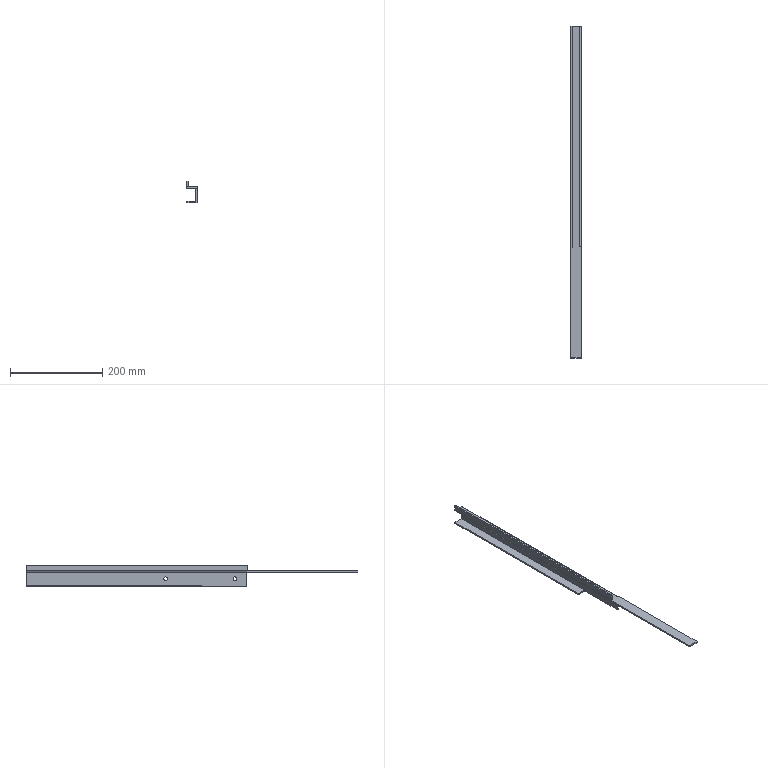Part | SolidWorks | features 3DProfileFeature 2, MirrorStock 1 | 1 solid | 46 faces | box 22.5 x 718.5 x 47 mm | volume 130417 mm3 | plane 36 | cylinder 10 | commonest cylinder face diameters 8 x4 0.4 x3 6.4 x3
STEP:
#1=CARTESIAN_POINT('',(19.5,393.,-10.5));
#2=VERTEX_POINT('',#1);
#3=CARTESIAN_POINT('',(19.5,393.,-18.5));
#4=VERTEX_POINT('',#3);
#5=CARTESIAN_POINT('',(19.5,393.,-14.5));
#6=DIRECTION('',(-1.,0.,0.));
#7=DIRECTION('',(0.,0.,1.));
#8=AXIS2_PLACEMENT_3D('',#5,#6,#7);
#9=CIRCLE('',#8,4.);
#10=EDGE_CURVE('',#2,#4,#9,.T.);
#11=ORIENTED_EDGE('',*,*,#10,.T.);
#12=CARTESIAN_POINT('',(22.5,393.,-18.5));
#13=VERTEX_POINT('',#12);
#14=CARTESIAN_POINT('',(19.5,393.,-18.5));
#15=DIRECTION('',(1.,0.,0.));
#16=VECTOR('',#15,1000.);
#17=LINE('',#14,#16);
#18=EDGE_CURVE('',#4,#13,#17,.T.);
#19=ORIENTED_EDGE('',*,*,#18,.T.);
#20=CARTESIAN_POINT('',(22.5,393.,-10.5));
#21=VERTEX_POINT('',#20);
#22=CARTESIAN_POINT('',(22.5,393.,-14.5));
#23=DIRECTION('',(-1.,0.,0.));
#24=DIRECTION('',(0.,0.,1.));
#25=AXIS2_PLACEMENT_3D('',#22,#23,#24);
#26=CIRCLE('',#25,4.);
#27=EDGE_CURVE('',#21,#13,#26,.T.);
#28=ORIENTED_EDGE('',*,*,#27,.F.);
#29=CARTESIAN_POINT('',(19.5,393.,-10.5));
#30=DIRECTION('',(1.,0.,0.));
#31=VECTOR('',#30,1000.);
#32=LINE('',#29,#31);
#33=EDGE_CURVE('',#2,#21,#32,.T.);
#34=ORIENTED_EDGE('',*,*,#33,.F.);
#35=EDGE_LOOP('',(#11,#19,#28,#34));
#36=FACE_OUTER_BOUND('',#35,.T.);
#37=CARTESIAN_POINT('',(19.5,393.,-14.5));
#38=DIRECTION('',(1.,0.,0.));
#39=DIRECTION('',(0.,0.,1.));
#40=AXIS2_PLACEMENT_3D('',#37,#38,#39);
#41=CYLINDRICAL_SURFACE('',#40,4.);
#42=ADVANCED_FACE('',(#36),#41,.F.);
#43=CARTESIAN_POINT('',(19.5,243.,-10.5));
#44=VERTEX_POINT('',#43);
#45=CARTESIAN_POINT('',(19.5,243.,-18.5));
#46=VERTEX_POINT('',#45);
#47=CARTESIAN_POINT('',(19.5,243.,-14.5));
#48=DIRECTION('',(-1.,0.,0.));
#49=DIRECTION('',(0.,0.,1.));
#50=AXIS2_PLACEMENT_3D('',#47,#48,#49);
#51=CIRCLE('',#50,4.);
#52=EDGE_CURVE('',#44,#46,#51,.T.);
#53=ORIENTED_EDGE('',*,*,#52,.T.);
#54=CARTESIAN_POINT('',(22.5,243.,-18.5));
#55=VERTEX_POINT('',#54);
#56=CARTESIAN_POINT('',(19.5,243.,-18.5));
#57=DIRECTION('',(1.,0.,0.));
#58=VECTOR('',#57,1000.);
#59=LINE('',#56,#58);
#60=EDGE_CURVE('',#46,#55,#59,.T.);
#61=ORIENTED_EDGE('',*,*,#60,.T.);
#62=CARTESIAN_POINT('',(22.5,243.,-10.5));
#63=VERTEX_POINT('',#62);
#64=CARTESIAN_POINT('',(22.5,243.,-14.5));
#65=DIRECTION('',(-1.,0.,0.));
#66=DIRECTION('',(0.,0.,1.));
#67=AXIS2_PLACEMENT_3D('',#64,#65,#66);
#68=CIRCLE('',#67,4.);
#69=EDGE_CURVE('',#63,#55,#68,.T.);
#70=ORIENTED_EDGE('',*,*,#69,.F.);
#71=CARTESIAN_POINT('',(19.5,243.,-10.5));
#72=DIRECTION('',(1.,0.,0.));
#73=VECTOR('',#72,1000.);
#74=LINE('',#71,#73);
#75=EDGE_CURVE('',#44,#63,#74,.T.);
#76=ORIENTED_EDGE('',*,*,#75,.F.);
#77=EDGE_LOOP('',(#53,#61,#70,#76));
#78=FACE_OUTER_BOUND('',#77,.T.);
#79=CARTESIAN_POINT('',(19.5,243.,-14.5));
#80=DIRECTION('',(1.,0.,0.));
#81=DIRECTION('',(0.,0.,1.));
#82=AXIS2_PLACEMENT_3D('',#79,#80,#81);
#83=CYLINDRICAL_SURFACE('',#82,4.);
#84=ADVANCED_FACE('',(#78),#83,.F.);
#85=CARTESIAN_POINT('',(19.3,695.,3.));
#86=VERTEX_POINT('',#85);
#87=CARTESIAN_POINT('',(3.2,695.,3.));
#88=VERTEX_POINT('',#87);
#89=CARTESIAN_POINT('',(0.,695.,3.));
#90=DIRECTION('',(-1.,0.,0.));
#91=VECTOR('',#90,1000.);
#92=LINE('',#89,#91);
#93=EDGE_CURVE('',#86,#88,#92,.T.);
#94=ORIENTED_EDGE('',*,*,#93,.F.);
#95=CARTESIAN_POINT('',(19.3,695.,0.));
#96=VERTEX_POINT('',#95);
#97=CARTESIAN_POINT('',(19.3,695.,0.));
#98=DIRECTION('',(0.,0.,1.));
#99=VECTOR('',#98,1000.);
#100=LINE('',#97,#99);
#101=EDGE_CURVE('',#96,#86,#100,.T.);
#102=ORIENTED_EDGE('',*,*,#101,.F.);
#103=CARTESIAN_POINT('',(3.2,695.,0.));
#104=VERTEX_POINT('',#103);
#105=CARTESIAN_POINT('',(0.,695.,0.));
#106=DIRECTION('',(-1.,0.,0.));
#107=VECTOR('',#106,1000.);
#108=LINE('',#105,#107);
#109=EDGE_CURVE('',#96,#104,#108,.T.);
#110=ORIENTED_EDGE('',*,*,#109,.T.);
#111=CARTESIAN_POINT('',(3.2,695.,3.));
#112=DIRECTION('',(0.,0.,-1.));
#113=VECTOR('',#112,1000.);
#114=LINE('',#111,#113);
#115=EDGE_CURVE('',#88,#104,#114,.T.);
#116=ORIENTED_EDGE('',*,*,#115,.F.);
#117=EDGE_LOOP('',(#94,#102,#110,#116));
#118=FACE_OUTER_BOUND('',#117,.T.);
#119=CARTESIAN_POINT('',(0.,695.,3.));
#120=DIRECTION('',(0.,1.,0.));
#121=DIRECTION('',(0.,0.,-1.));
#122=AXIS2_PLACEMENT_3D('',#119,#120,#121);
#123=PLANE('',#122);
#124=ADVANCED_FACE('',(#118),#123,.T.);
#125=CARTESIAN_POINT('',(3.2,216.5,3.));
#126=VERTEX_POINT('',#125);
#127=CARTESIAN_POINT('',(3.8,216.5,3.));
#128=VERTEX_POINT('',#127);
#129=CARTESIAN_POINT('',(3.2,216.5,3.));
#130=DIRECTION('',(1.,0.,0.));
#131=VECTOR('',#130,1000.);
#132=LINE('',#129,#131);
#133=EDGE_CURVE('',#126,#128,#132,.T.);
#134=ORIENTED_EDGE('',*,*,#133,.T.);
#135=CARTESIAN_POINT('',(3.8,215.9,3.));
#136=VERTEX_POINT('',#135);
#137=CARTESIAN_POINT('',(3.8,216.5,3.));
#138=DIRECTION('',(0.,-1.,0.));
#139=VECTOR('',#138,1000.);
#140=LINE('',#137,#139);
#141=EDGE_CURVE('',#128,#136,#140,.T.);
#142=ORIENTED_EDGE('',*,*,#141,.T.);
#143=CARTESIAN_POINT('',(0.,215.9,3.));
#144=VERTEX_POINT('',#143);
#145=CARTESIAN_POINT('',(3.8,215.9,3.));
#146=DIRECTION('',(-1.,0.,0.));
#147=VECTOR('',#146,1000.);
#148=LINE('',#145,#147);
#149=EDGE_CURVE('',#136,#144,#148,.T.);
#150=ORIENTED_EDGE('',*,*,#149,.T.);
#151=CARTESIAN_POINT('',(0.,-23.5,3.));
#152=VERTEX_POINT('',#151);
#153=CARTESIAN_POINT('',(0.,0.,3.));
#154=DIRECTION('',(0.,-1.,0.));
#155=VECTOR('',#154,1000.);
#156=LINE('',#153,#155);
#157=EDGE_CURVE('',#144,#152,#156,.T.);
#158=ORIENTED_EDGE('',*,*,#157,.T.);
#159=CARTESIAN_POINT('',(22.5,-23.5,3.));
#160=VERTEX_POINT('',#159);
#161=CARTESIAN_POINT('',(0.,-23.5,3.));
#162=DIRECTION('',(1.,0.,0.));
#163=VECTOR('',#162,1000.);
#164=LINE('',#161,#163);
#165=EDGE_CURVE('',#152,#160,#164,.T.);
#166=ORIENTED_EDGE('',*,*,#165,.T.);
#167=CARTESIAN_POINT('',(22.5,217.4,3.));
#168=VERTEX_POINT('',#167);
#169=CARTESIAN_POINT('',(22.5,0.,3.));
#170=DIRECTION('',(0.,1.,0.));
#171=VECTOR('',#170,1000.);
#172=LINE('',#169,#171);
#173=EDGE_CURVE('',#160,#168,#172,.T.);
#174=ORIENTED_EDGE('',*,*,#173,.T.);
#175=CARTESIAN_POINT('',(18.7,217.4,3.));
#176=VERTEX_POINT('',#175);
#177=CARTESIAN_POINT('',(0.,217.4,3.));
#178=DIRECTION('',(1.,0.,0.));
#179=VECTOR('',#178,1000.);
#180=LINE('',#177,#179);
#181=EDGE_CURVE('',#176,#168,#180,.T.);
#182=ORIENTED_EDGE('',*,*,#181,.F.);
#183=CARTESIAN_POINT('',(18.7,218.,3.));
#184=VERTEX_POINT('',#183);
#185=CARTESIAN_POINT('',(18.7,0.,3.));
#186=DIRECTION('',(0.,-1.,0.));
#187=VECTOR('',#186,1000.);
#188=LINE('',#185,#187);
#189=EDGE_CURVE('',#184,#176,#188,.T.);
#190=ORIENTED_EDGE('',*,*,#189,.F.);
#191=CARTESIAN_POINT('',(19.3,218.,3.));
#192=VERTEX_POINT('',#191);
#193=CARTESIAN_POINT('',(0.,218.,3.));
#194=DIRECTION('',(-1.,0.,0.));
#195=VECTOR('',#194,1000.);
#196=LINE('',#193,#195);
#197=EDGE_CURVE('',#192,#184,#196,.T.);
#198=ORIENTED_EDGE('',*,*,#197,.F.);
#199=CARTESIAN_POINT('',(19.3,695.,3.));
#200=DIRECTION('',(0.,-1.,0.));
#201=VECTOR('',#200,1000.);
#202=LINE('',#199,#201);
#203=EDGE_CURVE('',#86,#192,#202,.T.);
#204=ORIENTED_EDGE('',*,*,#203,.F.);
#205=ORIENTED_EDGE('',*,*,#93,.T.);
#206=CARTESIAN_POINT('',(3.2,695.,3.));
#207=DIRECTION('',(0.,-1.,0.));
#208=VECTOR('',#207,1000.);
#209=LINE('',#206,#208);
#210=EDGE_CURVE('',#88,#126,#209,.T.);
#211=ORIENTED_EDGE('',*,*,#210,.T.);
#212=EDGE_LOOP('',(#134,#142,#150,#158,#166,#174,#182,#190,#198,#204,#205,#211));
#213=FACE_OUTER_BOUND('',#212,.T.);
#214=CARTESIAN_POINT('',(0.,0.,3.));
#215=DIRECTION('',(0.,0.,1.));
#216=DIRECTION('',(-1.,0.,0.));
#217=AXIS2_PLACEMENT_3D('',#214,#215,#216);
#218=PLANE('',#217);
#219=ADVANCED_FACE('',(#213),#218,.T.);
#220=CARTESIAN_POINT('',(3.2,216.5,0.));
#221=VERTEX_POINT('',#220);
#222=CARTESIAN_POINT('',(3.2,695.,0.));
#223=DIRECTION('',(0.,-1.,0.));
#224=VECTOR('',#223,1000.);
#225=LINE('',#222,#224);
#226=EDGE_CURVE('',#104,#221,#225,.T.);
#227=ORIENTED_EDGE('',*,*,#226,.F.);
#228=ORIENTED_EDGE('',*,*,#109,.F.);
#229=CARTESIAN_POINT('',(19.3,218.,0.));
#230=VERTEX_POINT('',#229);
#231=CARTESIAN_POINT('',(19.3,695.,0.));
#232=DIRECTION('',(0.,-1.,0.));
#233=VECTOR('',#232,1000.);
#234=LINE('',#231,#233);
#235=EDGE_CURVE('',#96,#230,#234,.T.);
#236=ORIENTED_EDGE('',*,*,#235,.T.);
#237=CARTESIAN_POINT('',(18.7,218.,0.));
#238=VERTEX_POINT('',#237);
#239=CARTESIAN_POINT('',(19.3,218.,0.));
#240=DIRECTION('',(-1.,0.,0.));
#241=VECTOR('',#240,1000.);
#242=LINE('',#239,#241);
#243=EDGE_CURVE('',#230,#238,#242,.T.);
#244=ORIENTED_EDGE('',*,*,#243,.T.);
#245=CARTESIAN_POINT('',(18.7,217.4,0.));
#246=VERTEX_POINT('',#245);
#247=CARTESIAN_POINT('',(18.7,218.,0.));
#248=DIRECTION('',(0.,-1.,0.));
#249=VECTOR('',#248,1000.);
#250=LINE('',#247,#249);
#251=EDGE_CURVE('',#238,#246,#250,.T.);
#252=ORIENTED_EDGE('',*,*,#251,.T.);
#253=CARTESIAN_POINT('',(22.5,217.4,0.));
#254=VERTEX_POINT('',#253);
#255=CARTESIAN_POINT('',(18.7,217.4,0.));
#256=DIRECTION('',(1.,0.,0.));
#257=VECTOR('',#256,1000.);
#258=LINE('',#255,#257);
#259=EDGE_CURVE('',#246,#254,#258,.T.);
#260=ORIENTED_EDGE('',*,*,#259,.T.);
#261=CARTESIAN_POINT('',(22.5,-23.5,0.));
#262=VERTEX_POINT('',#261);
#263=CARTESIAN_POINT('',(22.5,0.,0.));
#264=DIRECTION('',(0.,1.,0.));
#265=VECTOR('',#264,1000.);
#266=LINE('',#263,#265);
#267=EDGE_CURVE('',#262,#254,#266,.T.);
#268=ORIENTED_EDGE('',*,*,#267,.F.);
#269=CARTESIAN_POINT('',(0.,-23.5,0.));
#270=VERTEX_POINT('',#269);
#271=CARTESIAN_POINT('',(22.5,-23.5,0.));
#272=DIRECTION('',(-1.,0.,0.));
#273=VECTOR('',#272,1000.);
#274=LINE('',#271,#273);
#275=EDGE_CURVE('',#262,#270,#274,.T.);
#276=ORIENTED_EDGE('',*,*,#275,.T.);
#277=CARTESIAN_POINT('',(0.,215.9,0.));
#278=VERTEX_POINT('',#277);
#279=CARTESIAN_POINT('',(0.,0.,0.));
#280=DIRECTION('',(0.,-1.,0.));
#281=VECTOR('',#280,1000.);
#282=LINE('',#279,#281);
#283=EDGE_CURVE('',#278,#270,#282,.T.);
#284=ORIENTED_EDGE('',*,*,#283,.F.);
#285=CARTESIAN_POINT('',(3.8,215.9,0.));
#286=VERTEX_POINT('',#285);
#287=CARTESIAN_POINT('',(0.,215.9,0.));
#288=DIRECTION('',(1.,0.,0.));
#289=VECTOR('',#288,1000.);
#290=LINE('',#287,#289);
#291=EDGE_CURVE('',#278,#286,#290,.T.);
#292=ORIENTED_EDGE('',*,*,#291,.T.);
#293=CARTESIAN_POINT('',(3.8,216.5,0.));
#294=VERTEX_POINT('',#293);
#295=CARTESIAN_POINT('',(3.8,0.,0.));
#296=DIRECTION('',(0.,1.,0.));
#297=VECTOR('',#296,1000.);
#298=LINE('',#295,#297);
#299=EDGE_CURVE('',#286,#294,#298,.T.);
#300=ORIENTED_EDGE('',*,*,#299,.T.);
#301=CARTESIAN_POINT('',(0.,216.5,0.));
#302=DIRECTION('',(-1.,0.,0.));
#303=VECTOR('',#302,1000.);
#304=LINE('',#301,#303);
#305=EDGE_CURVE('',#294,#221,#304,.T.);
#306=ORIENTED_EDGE('',*,*,#305,.T.);
#307=EDGE_LOOP('',(#227,#228,#236,#244,#252,#260,#268,#276,#284,#292,#300,#306));
#308=FACE_OUTER_BOUND('',#307,.T.);
#309=CARTESIAN_POINT('',(0.,0.,0.));
#310=DIRECTION('',(0.,0.,1.));
#311=DIRECTION('',(-1.,0.,0.));
#312=AXIS2_PLACEMENT_3D('',#309,#310,#311);
#313=PLANE('',#312);
#314=ADVANCED_FACE('',(#308),#313,.F.);
#315=ORIENTED_EDGE('',*,*,#283,.T.);
#316=CARTESIAN_POINT('',(0.,-23.5,0.));
#317=DIRECTION('',(0.,0.,1.));
#318=VECTOR('',#317,1000.);
#319=LINE('',#316,#318);
#320=EDGE_CURVE('',#270,#152,#319,.T.);
#321=ORIENTED_EDGE('',*,*,#320,.T.);
#322=ORIENTED_EDGE('',*,*,#157,.F.);
#323=CARTESIAN_POINT('',(0.,215.9,3.));
#324=DIRECTION('',(0.,0.,-1.));
#325=VECTOR('',#324,1000.);
#326=LINE('',#323,#325);
#327=EDGE_CURVE('',#144,#278,#326,.T.);
#328=ORIENTED_EDGE('',*,*,#327,.T.);
#329=EDGE_LOOP('',(#315,#321,#322,#328));
#330=FACE_OUTER_BOUND('',#329,.T.);
#331=CARTESIAN_POINT('',(0.,0.,3.));
#332=DIRECTION('',(-1.,0.,0.));
#333=DIRECTION('',(0.,0.,-1.));
#334=AXIS2_PLACEMENT_3D('',#331,#332,#333);
#335=PLANE('',#334);
#336=ADVANCED_FACE('',(#330),#335,.T.);
#337=CARTESIAN_POINT('',(19.5,695.,-28.8));
#338=VERTEX_POINT('',#337);
#339=CARTESIAN_POINT('',(19.5,695.,-0.2));
#340=VERTEX_POINT('',#339);
#341=CARTESIAN_POINT('',(19.5,695.,0.));
#342=DIRECTION('',(0.,0.,1.));
#343=VECTOR('',#342,1000.);
#344=LINE('',#341,#343);
#345=EDGE_CURVE('',#338,#340,#344,.T.);
#346=ORIENTED_EDGE('',*,*,#345,.T.);
#347=CARTESIAN_POINT('',(22.5,695.,-0.2));
#348=VERTEX_POINT('',#347);
#349=CARTESIAN_POINT('',(19.5,695.,-0.2));
#350=DIRECTION('',(1.,0.,0.));
#351=VECTOR('',#350,1000.);
#352=LINE('',#349,#351);
#353=EDGE_CURVE('',#340,#348,#352,.T.);
#354=ORIENTED_EDGE('',*,*,#353,.T.);
#355=CARTESIAN_POINT('',(22.5,695.,-28.8));
#356=VERTEX_POINT('',#355);
#357=CARTESIAN_POINT('',(22.5,695.,0.));
#358=DIRECTION('',(0.,0.,1.));
#359=VECTOR('',#358,1000.);
#360=LINE('',#357,#359);
#361=EDGE_CURVE('',#356,#348,#360,.T.);
#362=ORIENTED_EDGE('',*,*,#361,.F.);
#363=CARTESIAN_POINT('',(19.5,695.,-28.8));
#364=DIRECTION('',(1.,0.,0.));
#365=VECTOR('',#364,1000.);
#366=LINE('',#363,#365);
#367=EDGE_CURVE('',#338,#356,#366,.T.);
#368=ORIENTED_EDGE('',*,*,#367,.F.);
#369=EDGE_LOOP('',(#346,#354,#362,#368));
#370=FACE_OUTER_BOUND('',#369,.T.);
#371=CARTESIAN_POINT('',(22.5,695.,0.));
#372=DIRECTION('',(0.,1.,0.));
#373=DIRECTION('',(0.,0.,-1.));
#374=AXIS2_PLACEMENT_3D('',#371,#372,#373);
#375=PLANE('',#374);
#376=ADVANCED_FACE('',(#370),#375,.T.);
#377=ORIENTED_EDGE('',*,*,#27,.T.);
#378=CARTESIAN_POINT('',(22.5,393.,-14.5));
#379=DIRECTION('',(-1.,0.,0.));
#380=DIRECTION('',(0.,0.,1.));
#381=AXIS2_PLACEMENT_3D('',#378,#379,#380);
#382=CIRCLE('',#381,4.);
#383=EDGE_CURVE('',#13,#21,#382,.T.);
#384=ORIENTED_EDGE('',*,*,#383,.T.);
#385=EDGE_LOOP('',(#377,#384));
#386=FACE_BOUND('',#385,.T.);
#387=ORIENTED_EDGE('',*,*,#69,.T.);
#388=CARTESIAN_POINT('',(22.5,243.,-14.5));
#389=DIRECTION('',(-1.,0.,0.));
#390=DIRECTION('',(0.,0.,1.));
#391=AXIS2_PLACEMENT_3D('',#388,#389,#390);
#392=CIRCLE('',#391,4.);
#393=EDGE_CURVE('',#55,#63,#392,.T.);
#394=ORIENTED_EDGE('',*,*,#393,.T.);
#395=EDGE_LOOP('',(#387,#394));
#396=FACE_BOUND('',#395,.T.);
#397=ORIENTED_EDGE('',*,*,#361,.T.);
#398=CARTESIAN_POINT('',(22.5,218.,-0.2));
#399=VERTEX_POINT('',#398);
#400=CARTESIAN_POINT('',(22.5,0.,-0.2));
#401=DIRECTION('',(0.,1.,0.));
#402=VECTOR('',#401,1000.);
#403=LINE('',#400,#402);
#404=EDGE_CURVE('',#399,#348,#403,.T.);
#405=ORIENTED_EDGE('',*,*,#404,.F.);
#406=CARTESIAN_POINT('',(22.5,218.,-32.));
#407=VERTEX_POINT('',#406);
#408=CARTESIAN_POINT('',(22.5,218.,-32.));
#409=DIRECTION('',(0.,0.,-1.));
#410=VECTOR('',#409,1000.);
#411=LINE('',#408,#410);
#412=EDGE_CURVE('',#399,#407,#411,.T.);
#413=ORIENTED_EDGE('',*,*,#412,.T.);
#414=CARTESIAN_POINT('',(22.5,315.9,-32.));
#415=VERTEX_POINT('',#414);
#416=CARTESIAN_POINT('',(22.5,695.,-32.));
#417=DIRECTION('',(0.,1.,0.));
#418=VECTOR('',#417,1000.);
#419=LINE('',#416,#418);
#420=EDGE_CURVE('',#407,#415,#419,.T.);
#421=ORIENTED_EDGE('',*,*,#420,.T.);
#422=CARTESIAN_POINT('',(22.5,315.9,-28.2));
#423=VERTEX_POINT('',#422);
#424=CARTESIAN_POINT('',(22.5,315.9,0.));
#425=DIRECTION('',(0.,0.,-1.));
#426=VECTOR('',#425,1000.);
#427=LINE('',#424,#426);
#428=EDGE_CURVE('',#423,#415,#427,.T.);
#429=ORIENTED_EDGE('',*,*,#428,.F.);
#430=CARTESIAN_POINT('',(22.5,316.5,-28.2));
#431=VERTEX_POINT('',#430);
#432=CARTESIAN_POINT('',(22.5,0.,-28.2));
#433=DIRECTION('',(0.,-1.,0.));
#434=VECTOR('',#433,1000.);
#435=LINE('',#432,#434);
#436=EDGE_CURVE('',#431,#423,#435,.T.);
#437=ORIENTED_EDGE('',*,*,#436,.F.);
#438=CARTESIAN_POINT('',(22.5,316.5,-28.8));
#439=VERTEX_POINT('',#438);
#440=CARTESIAN_POINT('',(22.5,316.5,0.));
#441=DIRECTION('',(0.,0.,1.));
#442=VECTOR('',#441,1000.);
#443=LINE('',#440,#442);
#444=EDGE_CURVE('',#439,#431,#443,.T.);
#445=ORIENTED_EDGE('',*,*,#444,.F.);
#446=CARTESIAN_POINT('',(22.5,695.,-28.8));
#447=DIRECTION('',(0.,-1.,0.));
#448=VECTOR('',#447,1000.);
#449=LINE('',#446,#448);
#450=EDGE_CURVE('',#356,#439,#449,.T.);
#451=ORIENTED_EDGE('',*,*,#450,.F.);
#452=EDGE_LOOP('',(#397,#405,#413,#421,#429,#437,#445,#451));
#453=FACE_OUTER_BOUND('',#452,.T.);
#454=CARTESIAN_POINT('',(22.5,0.,0.));
#455=DIRECTION('',(1.,0.,0.));
#456=DIRECTION('',(0.,0.,1.));
#457=AXIS2_PLACEMENT_3D('',#454,#455,#456);
#458=PLANE('',#457);
#459=ADVANCED_FACE('',(#386,#396,#453),#458,.T.);
#460=ORIENTED_EDGE('',*,*,#10,.F.);
#461=CARTESIAN_POINT('',(19.5,393.,-14.5));
#462=DIRECTION('',(-1.,0.,0.));
#463=DIRECTION('',(0.,0.,1.));
#464=AXIS2_PLACEMENT_3D('',#461,#462,#463);
#465=CIRCLE('',#464,4.);
#466=EDGE_CURVE('',#4,#2,#465,.T.);
#467=ORIENTED_EDGE('',*,*,#466,.F.);
#468=EDGE_LOOP('',(#460,#467));
#469=FACE_BOUND('',#468,.T.);
#470=ORIENTED_EDGE('',*,*,#52,.F.);
#471=CARTESIAN_POINT('',(19.5,243.,-14.5));
#472=DIRECTION('',(-1.,0.,0.));
#473=DIRECTION('',(0.,0.,1.));
#474=AXIS2_PLACEMENT_3D('',#471,#472,#473);
#475=CIRCLE('',#474,4.);
#476=EDGE_CURVE('',#46,#44,#475,.T.);
#477=ORIENTED_EDGE('',*,*,#476,.F.);
#478=EDGE_LOOP('',(#470,#477));
#479=FACE_BOUND('',#478,.T.);
#480=CARTESIAN_POINT('',(19.5,316.5,-28.8));
#481=VERTEX_POINT('',#480);
#482=CARTESIAN_POINT('',(19.5,695.,-28.8));
#483=DIRECTION('',(0.,-1.,0.));
#484=VECTOR('',#483,1000.);
#485=LINE('',#482,#484);
#486=EDGE_CURVE('',#338,#481,#485,.T.);
#487=ORIENTED_EDGE('',*,*,#486,.T.);
#488=CARTESIAN_POINT('',(19.5,316.5,-28.2));
#489=VERTEX_POINT('',#488);
#490=CARTESIAN_POINT('',(19.5,316.5,-28.8));
#491=DIRECTION('',(0.,0.,1.));
#492=VECTOR('',#491,1000.);
#493=LINE('',#490,#492);
#494=EDGE_CURVE('',#481,#489,#493,.T.);
#495=ORIENTED_EDGE('',*,*,#494,.T.);
#496=CARTESIAN_POINT('',(19.5,315.9,-28.2));
#497=VERTEX_POINT('',#496);
#498=CARTESIAN_POINT('',(19.5,316.5,-28.2));
#499=DIRECTION('',(0.,-1.,0.));
#500=VECTOR('',#499,1000.);
#501=LINE('',#498,#500);
#502=EDGE_CURVE('',#489,#497,#501,.T.);
#503=ORIENTED_EDGE('',*,*,#502,.T.);
#504=CARTESIAN_POINT('',(19.5,315.9,-32.));
#505=VERTEX_POINT('',#504);
#506=CARTESIAN_POINT('',(19.5,315.9,-28.2));
#507=DIRECTION('',(0.,0.,-1.));
#508=VECTOR('',#507,1000.);
#509=LINE('',#506,#508);
#510=EDGE_CURVE('',#497,#505,#509,.T.);
#511=ORIENTED_EDGE('',*,*,#510,.T.);
#512=CARTESIAN_POINT('',(19.5,218.,-32.));
#513=VERTEX_POINT('',#512);
#514=CARTESIAN_POINT('',(19.5,0.,-32.));
#515=DIRECTION('',(0.,1.,0.));
#516=VECTOR('',#515,1000.);
#517=LINE('',#514,#516);
#518=EDGE_CURVE('',#513,#505,#517,.T.);
#519=ORIENTED_EDGE('',*,*,#518,.F.);
#520=CARTESIAN_POINT('',(19.5,218.,-0.2));
#521=VERTEX_POINT('',#520);
#522=CARTESIAN_POINT('',(19.5,218.,0.));
#523=DIRECTION('',(0.,0.,-1.));
#524=VECTOR('',#523,1000.);
#525=LINE('',#522,#524);
#526=EDGE_CURVE('',#521,#513,#525,.T.);
#527=ORIENTED_EDGE('',*,*,#526,.F.);
#528=CARTESIAN_POINT('',(19.5,218.,-0.2));
#529=DIRECTION('',(0.,1.,0.));
#530=VECTOR('',#529,1000.);
#531=LINE('',#528,#530);
#532=EDGE_CURVE('',#521,#340,#531,.T.);
#533=ORIENTED_EDGE('',*,*,#532,.T.);
#534=ORIENTED_EDGE('',*,*,#345,.F.);
#535=EDGE_LOOP('',(#487,#495,#503,#511,#519,#527,#533,#534));
#536=FACE_OUTER_BOUND('',#535,.T.);
#537=CARTESIAN_POINT('',(19.5,0.,0.));
#538=DIRECTION('',(1.,0.,0.));
#539=DIRECTION('',(0.,0.,1.));
#540=AXIS2_PLACEMENT_3D('',#537,#538,#539);
#541=PLANE('',#540);
#542=ADVANCED_FACE('',(#469,#479,#536),#541,.F.);
#543=ORIENTED_EDGE('',*,*,#420,.F.);
#544=CARTESIAN_POINT('',(22.5,218.,-32.));
#545=DIRECTION('',(-1.,0.,0.));
#546=VECTOR('',#545,1000.);
#547=LINE('',#544,#546);
#548=EDGE_CURVE('',#407,#513,#547,.T.);
#549=ORIENTED_EDGE('',*,*,#548,.T.);
#550=ORIENTED_EDGE('',*,*,#518,.T.);
#551=CARTESIAN_POINT('',(19.5,315.9,-32.));
#552=DIRECTION('',(1.,0.,0.));
#553=VECTOR('',#552,1000.);
#554=LINE('',#551,#553);
#555=EDGE_CURVE('',#505,#415,#554,.T.);
#556=ORIENTED_EDGE('',*,*,#555,.T.);
#557=EDGE_LOOP('',(#543,#549,#550,#556));
#558=FACE_OUTER_BOUND('',#557,.T.);
#559=CARTESIAN_POINT('',(22.5,695.,-32.));
#560=DIRECTION('',(0.,0.,-1.));
#561=DIRECTION('',(1.,0.,0.));
#562=AXIS2_PLACEMENT_3D('',#559,#560,#561);
#563=PLANE('',#562);
#564=ADVANCED_FACE('',(#558),#563,.T.);
#565=ORIENTED_EDGE('',*,*,#173,.F.);
#566=CARTESIAN_POINT('',(22.5,-23.5,3.));
#567=DIRECTION('',(0.,0.,-1.));
#568=VECTOR('',#567,1000.);
#569=LINE('',#566,#568);
#570=EDGE_CURVE('',#160,#262,#569,.T.);
#571=ORIENTED_EDGE('',*,*,#570,.T.);
#572=ORIENTED_EDGE('',*,*,#267,.T.);
#573=CARTESIAN_POINT('',(22.5,217.4,0.));
#574=DIRECTION('',(0.,0.,1.));
#575=VECTOR('',#574,1000.);
#576=LINE('',#573,#575);
#577=EDGE_CURVE('',#254,#168,#576,.T.);
#578=ORIENTED_EDGE('',*,*,#577,.T.);
#579=EDGE_LOOP('',(#565,#571,#572,#578));
#580=FACE_OUTER_BOUND('',#579,.T.);
#581=CARTESIAN_POINT('',(22.5,0.,3.));
#582=DIRECTION('',(1.,0.,0.));
#583=DIRECTION('',(0.,0.,1.));
#584=AXIS2_PLACEMENT_3D('',#581,#582,#583);
#585=PLANE('',#584);
#586=ADVANCED_FACE('',(#580),#585,.T.);
#587=ORIENTED_EDGE('',*,*,#197,.T.);
#588=CARTESIAN_POINT('',(18.7,218.,0.));
#589=DIRECTION('',(0.,0.,1.));
#590=VECTOR('',#589,1000.);
#591=LINE('',#588,#590);
#592=EDGE_CURVE('',#238,#184,#591,.T.);
#593=ORIENTED_EDGE('',*,*,#592,.F.);
#594=ORIENTED_EDGE('',*,*,#243,.F.);
#595=CARTESIAN_POINT('',(19.3,218.,0.));
#596=DIRECTION('',(0.,0.,1.));
#597=VECTOR('',#596,1000.);
#598=LINE('',#595,#597);
#599=EDGE_CURVE('',#230,#192,#598,.T.);
#600=ORIENTED_EDGE('',*,*,#599,.T.);
#601=EDGE_LOOP('',(#587,#593,#594,#600));
#602=FACE_OUTER_BOUND('',#601,.T.);
#603=CARTESIAN_POINT('',(19.3,218.,0.));
#604=DIRECTION('',(0.,-1.,0.));
#605=DIRECTION('',(0.,0.,1.));
#606=AXIS2_PLACEMENT_3D('',#603,#604,#605);
#607=PLANE('',#606);
#608=ADVANCED_FACE('',(#602),#607,.T.);
#609=ORIENTED_EDGE('',*,*,#189,.T.);
#610=CARTESIAN_POINT('',(18.7,217.4,0.));
#611=DIRECTION('',(0.,0.,1.));
#612=VECTOR('',#611,1000.);
#613=LINE('',#610,#612);
#614=EDGE_CURVE('',#246,#176,#613,.T.);
#615=ORIENTED_EDGE('',*,*,#614,.F.);
#616=ORIENTED_EDGE('',*,*,#251,.F.);
#617=ORIENTED_EDGE('',*,*,#592,.T.);
#618=EDGE_LOOP('',(#609,#615,#616,#617));
#619=FACE_OUTER_BOUND('',#618,.T.);
#620=CARTESIAN_POINT('',(18.7,218.,0.));
#621=DIRECTION('',(1.,0.,0.));
#622=DIRECTION('',(0.,0.,1.));
#623=AXIS2_PLACEMENT_3D('',#620,#621,#622);
#624=PLANE('',#623);
#625=ADVANCED_FACE('',(#619),#624,.T.);
#626=ORIENTED_EDGE('',*,*,#181,.T.);
#627=ORIENTED_EDGE('',*,*,#577,.F.);
#628=ORIENTED_EDGE('',*,*,#259,.F.);
#629=ORIENTED_EDGE('',*,*,#614,.T.);
#630=EDGE_LOOP('',(#626,#627,#628,#629));
#631=FACE_OUTER_BOUND('',#630,.T.);
#632=CARTESIAN_POINT('',(18.7,217.4,0.));
#633=DIRECTION('',(0.,1.,0.));
#634=DIRECTION('',(0.,0.,-1.));
#635=AXIS2_PLACEMENT_3D('',#632,#633,#634);
#636=PLANE('',#635);
#637=ADVANCED_FACE('',(#631),#636,.T.);
#638=CARTESIAN_POINT('',(22.5,218.,-0.2));
#639=DIRECTION('',(1.,0.,0.));
#640=VECTOR('',#639,1000.);
#641=LINE('',#638,#640);
#642=EDGE_CURVE('',#521,#399,#641,.T.);
#643=ORIENTED_EDGE('',*,*,#642,.T.);
#644=CARTESIAN_POINT('',(19.3,218.,-0.2));
#645=DIRECTION('',(0.,1.,0.));
#646=DIRECTION('',(0.,0.,-1.));
#647=AXIS2_PLACEMENT_3D('',#644,#645,#646);
#648=CIRCLE('',#647,3.2);
#649=EDGE_CURVE('',#192,#399,#648,.T.);
#650=ORIENTED_EDGE('',*,*,#649,.F.);
#651=ORIENTED_EDGE('',*,*,#599,.F.);
#652=CARTESIAN_POINT('',(19.3,218.,-0.2));
#653=DIRECTION('',(0.,1.,0.));
#654=DIRECTION('',(0.,0.,-1.));
#655=AXIS2_PLACEMENT_3D('',#652,#653,#654);
#656=CIRCLE('',#655,0.2);
#657=EDGE_CURVE('',#230,#521,#656,.T.);
#658=ORIENTED_EDGE('',*,*,#657,.T.);
#659=EDGE_LOOP('',(#643,#650,#651,#658));
#660=FACE_OUTER_BOUND('',#659,.T.);
#661=CARTESIAN_POINT('',(19.3,218.,-0.2));
#662=DIRECTION('',(0.,-1.,0.));
#663=DIRECTION('',(0.,0.,1.));
#664=AXIS2_PLACEMENT_3D('',#661,#662,#663);
#665=PLANE('',#664);
#666=ADVANCED_FACE('',(#660),#665,.T.);
#667=CARTESIAN_POINT('',(19.3,695.,-0.2));
#668=DIRECTION('',(0.,-1.,0.));
#669=DIRECTION('',(0.,0.,-1.));
#670=AXIS2_PLACEMENT_3D('',#667,#668,#669);
#671=CIRCLE('',#670,0.2);
#672=EDGE_CURVE('',#340,#96,#671,.T.);
#673=ORIENTED_EDGE('',*,*,#672,.T.);
#674=ORIENTED_EDGE('',*,*,#101,.T.);
#675=CARTESIAN_POINT('',(19.3,695.,-0.2));
#676=DIRECTION('',(0.,-1.,0.));
#677=DIRECTION('',(0.,0.,-1.));
#678=AXIS2_PLACEMENT_3D('',#675,#676,#677);
#679=CIRCLE('',#678,3.2);
#680=EDGE_CURVE('',#348,#86,#679,.T.);
#681=ORIENTED_EDGE('',*,*,#680,.F.);
#682=ORIENTED_EDGE('',*,*,#353,.F.);
#683=EDGE_LOOP('',(#673,#674,#681,#682));
#684=FACE_OUTER_BOUND('',#683,.T.);
#685=CARTESIAN_POINT('',(19.3,695.,-0.2));
#686=DIRECTION('',(0.,-1.,0.));
#687=DIRECTION('',(0.,0.,1.));
#688=AXIS2_PLACEMENT_3D('',#685,#686,#687);
#689=PLANE('',#688);
#690=ADVANCED_FACE('',(#684),#689,.F.);
#691=ORIENTED_EDGE('',*,*,#203,.T.);
#692=ORIENTED_EDGE('',*,*,#649,.T.);
#693=ORIENTED_EDGE('',*,*,#404,.T.);
#694=ORIENTED_EDGE('',*,*,#680,.T.);
#695=EDGE_LOOP('',(#691,#692,#693,#694));
#696=FACE_OUTER_BOUND('',#695,.T.);
#697=CARTESIAN_POINT('',(19.3,695.,-0.2));
#698=DIRECTION('',(0.,1.,0.));
#699=DIRECTION('',(1.,0.,0.));
#700=AXIS2_PLACEMENT_3D('',#697,#698,#699);
#701=CYLINDRICAL_SURFACE('',#700,3.2);
#702=ADVANCED_FACE('',(#696),#701,.T.);
#703=ORIENTED_EDGE('',*,*,#235,.F.);
#704=ORIENTED_EDGE('',*,*,#672,.F.);
#705=ORIENTED_EDGE('',*,*,#532,.F.);
#706=ORIENTED_EDGE('',*,*,#657,.F.);
#707=EDGE_LOOP('',(#703,#704,#705,#706));
#708=FACE_OUTER_BOUND('',#707,.T.);
#709=CARTESIAN_POINT('',(19.3,695.,-0.2));
#710=DIRECTION('',(0.,1.,0.));
#711=DIRECTION('',(1.,0.,0.));
#712=AXIS2_PLACEMENT_3D('',#709,#710,#711);
#713=CYLINDRICAL_SURFACE('',#712,0.2);
#714=ADVANCED_FACE('',(#708),#713,.F.);
#715=ORIENTED_EDGE('',*,*,#526,.T.);
#716=ORIENTED_EDGE('',*,*,#548,.F.);
#717=ORIENTED_EDGE('',*,*,#412,.F.);
#718=ORIENTED_EDGE('',*,*,#642,.F.);
#719=EDGE_LOOP('',(#715,#716,#717,#718));
#720=FACE_OUTER_BOUND('',#719,.T.);
#721=CARTESIAN_POINT('',(22.5,218.,-32.));
#722=DIRECTION('',(0.,-1.,0.));
#723=DIRECTION('',(0.,0.,1.));
#724=AXIS2_PLACEMENT_3D('',#721,#722,#723);
#725=PLANE('',#724);
#726=ADVANCED_FACE('',(#720),#725,.T.);
#727=ORIENTED_EDGE('',*,*,#444,.T.);
#728=CARTESIAN_POINT('',(19.5,316.5,-28.2));
#729=DIRECTION('',(1.,0.,0.));
#730=VECTOR('',#729,1000.);
#731=LINE('',#728,#730);
#732=EDGE_CURVE('',#489,#431,#731,.T.);
#733=ORIENTED_EDGE('',*,*,#732,.F.);
#734=ORIENTED_EDGE('',*,*,#494,.F.);
#735=CARTESIAN_POINT('',(19.5,316.5,-28.8));
#736=DIRECTION('',(1.,0.,0.));
#737=VECTOR('',#736,1000.);
#738=LINE('',#735,#737);
#739=EDGE_CURVE('',#481,#439,#738,.T.);
#740=ORIENTED_EDGE('',*,*,#739,.T.);
#741=EDGE_LOOP('',(#727,#733,#734,#740));
#742=FACE_OUTER_BOUND('',#741,.T.);
#743=CARTESIAN_POINT('',(19.5,316.5,-28.8));
#744=DIRECTION('',(0.,-1.,0.));
#745=DIRECTION('',(1.,0.,0.));
#746=AXIS2_PLACEMENT_3D('',#743,#744,#745);
#747=PLANE('',#746);
#748=ADVANCED_FACE('',(#742),#747,.T.);
#749=ORIENTED_EDGE('',*,*,#436,.T.);
#750=CARTESIAN_POINT('',(19.5,315.9,-28.2));
#751=DIRECTION('',(1.,0.,0.));
#752=VECTOR('',#751,1000.);
#753=LINE('',#750,#752);
#754=EDGE_CURVE('',#497,#423,#753,.T.);
#755=ORIENTED_EDGE('',*,*,#754,.F.);
#756=ORIENTED_EDGE('',*,*,#502,.F.);
#757=ORIENTED_EDGE('',*,*,#732,.T.);
#758=EDGE_LOOP('',(#749,#755,#756,#757));
#759=FACE_OUTER_BOUND('',#758,.T.);
#760=CARTESIAN_POINT('',(19.5,316.5,-28.2));
#761=DIRECTION('',(0.,0.,-1.));
#762=DIRECTION('',(1.,0.,0.));
#763=AXIS2_PLACEMENT_3D('',#760,#761,#762);
#764=PLANE('',#763);
#765=ADVANCED_FACE('',(#759),#764,.T.);
#766=ORIENTED_EDGE('',*,*,#428,.T.);
#767=ORIENTED_EDGE('',*,*,#555,.F.);
#768=ORIENTED_EDGE('',*,*,#510,.F.);
#769=ORIENTED_EDGE('',*,*,#754,.T.);
#770=EDGE_LOOP('',(#766,#767,#768,#769));
#771=FACE_OUTER_BOUND('',#770,.T.);
#772=CARTESIAN_POINT('',(19.5,315.9,-28.2));
#773=DIRECTION('',(0.,1.,0.));
#774=DIRECTION('',(-1.,0.,0.));
#775=AXIS2_PLACEMENT_3D('',#772,#773,#774);
#776=PLANE('',#775);
#777=ADVANCED_FACE('',(#771),#776,.T.);
#778=CARTESIAN_POINT('',(19.3,316.5,-29.));
#779=VERTEX_POINT('',#778);
#780=CARTESIAN_POINT('',(19.3,316.5,-32.));
#781=VERTEX_POINT('',#780);
#782=CARTESIAN_POINT('',(19.3,316.5,-32.));
#783=DIRECTION('',(0.,0.,-1.));
#784=VECTOR('',#783,1000.);
#785=LINE('',#782,#784);
#786=EDGE_CURVE('',#779,#781,#785,.T.);
#787=ORIENTED_EDGE('',*,*,#786,.T.);
#788=CARTESIAN_POINT('',(19.3,316.5,-28.8));
#789=DIRECTION('',(0.,1.,0.));
#790=DIRECTION('',(0.,0.,-1.));
#791=AXIS2_PLACEMENT_3D('',#788,#789,#790);
#792=CIRCLE('',#791,3.2);
#793=EDGE_CURVE('',#439,#781,#792,.T.);
#794=ORIENTED_EDGE('',*,*,#793,.F.);
#795=ORIENTED_EDGE('',*,*,#739,.F.);
#796=CARTESIAN_POINT('',(19.3,316.5,-28.8));
#797=DIRECTION('',(0.,1.,0.));
#798=DIRECTION('',(0.,0.,-1.));
#799=AXIS2_PLACEMENT_3D('',#796,#797,#798);
#800=CIRCLE('',#799,0.2);
#801=EDGE_CURVE('',#481,#779,#800,.T.);
#802=ORIENTED_EDGE('',*,*,#801,.T.);
#803=EDGE_LOOP('',(#787,#794,#795,#802));
#804=FACE_OUTER_BOUND('',#803,.T.);
#805=CARTESIAN_POINT('',(19.3,316.5,-28.8));
#806=DIRECTION('',(0.,-1.,0.));
#807=DIRECTION('',(0.,0.,1.));
#808=AXIS2_PLACEMENT_3D('',#805,#806,#807);
#809=PLANE('',#808);
#810=ADVANCED_FACE('',(#804),#809,.T.);
#811=CARTESIAN_POINT('',(19.3,695.,-29.));
#812=VERTEX_POINT('',#811);
#813=CARTESIAN_POINT('',(19.3,695.,-28.8));
#814=DIRECTION('',(0.,-1.,0.));
#815=DIRECTION('',(0.,0.,-1.));
#816=AXIS2_PLACEMENT_3D('',#813,#814,#815);
#817=CIRCLE('',#816,0.2);
#818=EDGE_CURVE('',#812,#338,#817,.T.);
#819=ORIENTED_EDGE('',*,*,#818,.T.);
#820=ORIENTED_EDGE('',*,*,#367,.T.);
#821=CARTESIAN_POINT('',(19.3,695.,-32.));
#822=VERTEX_POINT('',#821);
#823=CARTESIAN_POINT('',(19.3,695.,-28.8));
#824=DIRECTION('',(0.,-1.,0.));
#825=DIRECTION('',(0.,0.,-1.));
#826=AXIS2_PLACEMENT_3D('',#823,#824,#825);
#827=CIRCLE('',#826,3.2);
#828=EDGE_CURVE('',#822,#356,#827,.T.);
#829=ORIENTED_EDGE('',*,*,#828,.F.);
#830=CARTESIAN_POINT('',(19.3,695.,-29.));
#831=DIRECTION('',(0.,0.,-1.));
#832=VECTOR('',#831,1000.);
#833=LINE('',#830,#832);
#834=EDGE_CURVE('',#812,#822,#833,.T.);
#835=ORIENTED_EDGE('',*,*,#834,.F.);
#836=EDGE_LOOP('',(#819,#820,#829,#835));
#837=FACE_OUTER_BOUND('',#836,.T.);
#838=CARTESIAN_POINT('',(19.3,695.,-28.8));
#839=DIRECTION('',(0.,-1.,0.));
#840=DIRECTION('',(0.,0.,1.));
#841=AXIS2_PLACEMENT_3D('',#838,#839,#840);
#842=PLANE('',#841);
#843=ADVANCED_FACE('',(#837),#842,.F.);
#844=ORIENTED_EDGE('',*,*,#450,.T.);
#845=ORIENTED_EDGE('',*,*,#793,.T.);
#846=CARTESIAN_POINT('',(19.3,0.,-32.));
#847=DIRECTION('',(0.,1.,0.));
#848=VECTOR('',#847,1000.);
#849=LINE('',#846,#848);
#850=EDGE_CURVE('',#781,#822,#849,.T.);
#851=ORIENTED_EDGE('',*,*,#850,.T.);
#852=ORIENTED_EDGE('',*,*,#828,.T.);
#853=EDGE_LOOP('',(#844,#845,#851,#852));
#854=FACE_OUTER_BOUND('',#853,.T.);
#855=CARTESIAN_POINT('',(19.3,695.,-28.8));
#856=DIRECTION('',(0.,1.,0.));
#857=DIRECTION('',(0.,0.,-1.));
#858=AXIS2_PLACEMENT_3D('',#855,#856,#857);
#859=CYLINDRICAL_SURFACE('',#858,3.2);
#860=ADVANCED_FACE('',(#854),#859,.T.);
#861=ORIENTED_EDGE('',*,*,#486,.F.);
#862=ORIENTED_EDGE('',*,*,#818,.F.);
#863=CARTESIAN_POINT('',(19.3,316.5,-29.));
#864=DIRECTION('',(0.,1.,0.));
#865=VECTOR('',#864,1000.);
#866=LINE('',#863,#865);
#867=EDGE_CURVE('',#779,#812,#866,.T.);
#868=ORIENTED_EDGE('',*,*,#867,.F.);
#869=ORIENTED_EDGE('',*,*,#801,.F.);
#870=EDGE_LOOP('',(#861,#862,#868,#869));
#871=FACE_OUTER_BOUND('',#870,.T.);
#872=CARTESIAN_POINT('',(19.3,695.,-28.8));
#873=DIRECTION('',(0.,1.,0.));
#874=DIRECTION('',(0.,0.,-1.));
#875=AXIS2_PLACEMENT_3D('',#872,#873,#874);
#876=CYLINDRICAL_SURFACE('',#875,0.2);
#877=ADVANCED_FACE('',(#871),#876,.F.);
#878=CARTESIAN_POINT('',(0.,695.,-32.));
#879=VERTEX_POINT('',#878);
#880=CARTESIAN_POINT('',(19.5,695.,-32.));
#881=DIRECTION('',(1.,0.,0.));
#882=VECTOR('',#881,1000.);
#883=LINE('',#880,#882);
#884=EDGE_CURVE('',#879,#822,#883,.T.);
#885=ORIENTED_EDGE('',*,*,#884,.F.);
#886=CARTESIAN_POINT('',(0.,695.,-29.));
#887=VERTEX_POINT('',#886);
#888=CARTESIAN_POINT('',(0.,695.,-32.));
#889=DIRECTION('',(0.,0.,1.));
#890=VECTOR('',#889,1000.);
#891=LINE('',#888,#890);
#892=EDGE_CURVE('',#879,#887,#891,.T.);
#893=ORIENTED_EDGE('',*,*,#892,.T.);
#894=CARTESIAN_POINT('',(0.,695.,-29.));
#895=DIRECTION('',(1.,0.,0.));
#896=VECTOR('',#895,1000.);
#897=LINE('',#894,#896);
#898=EDGE_CURVE('',#887,#812,#897,.T.);
#899=ORIENTED_EDGE('',*,*,#898,.T.);
#900=ORIENTED_EDGE('',*,*,#834,.T.);
#901=EDGE_LOOP('',(#885,#893,#899,#900));
#902=FACE_OUTER_BOUND('',#901,.T.);
#903=CARTESIAN_POINT('',(19.5,695.,-32.));
#904=DIRECTION('',(0.,1.,0.));
#905=DIRECTION('',(0.,0.,-1.));
#906=AXIS2_PLACEMENT_3D('',#903,#904,#905);
#907=PLANE('',#906);
#908=ADVANCED_FACE('',(#902),#907,.T.);
#909=CARTESIAN_POINT('',(0.,316.5,-29.));
#910=VERTEX_POINT('',#909);
#911=CARTESIAN_POINT('',(0.,316.5,-29.));
#912=DIRECTION('',(-1.,0.,0.));
#913=VECTOR('',#912,1000.);
#914=LINE('',#911,#913);
#915=EDGE_CURVE('',#779,#910,#914,.T.);
#916=ORIENTED_EDGE('',*,*,#915,.T.);
#917=CARTESIAN_POINT('',(0.,316.5,-32.));
#918=VERTEX_POINT('',#917);
#919=CARTESIAN_POINT('',(0.,316.5,-32.));
#920=DIRECTION('',(0.,0.,1.));
#921=VECTOR('',#920,1000.);
#922=LINE('',#919,#921);
#923=EDGE_CURVE('',#918,#910,#922,.T.);
#924=ORIENTED_EDGE('',*,*,#923,.F.);
#925=CARTESIAN_POINT('',(0.,316.5,-32.));
#926=DIRECTION('',(-1.,0.,0.));
#927=VECTOR('',#926,1000.);
#928=LINE('',#925,#927);
#929=EDGE_CURVE('',#781,#918,#928,.T.);
#930=ORIENTED_EDGE('',*,*,#929,.F.);
#931=ORIENTED_EDGE('',*,*,#786,.F.);
#932=EDGE_LOOP('',(#916,#924,#930,#931));
#933=FACE_OUTER_BOUND('',#932,.T.);
#934=CARTESIAN_POINT('',(0.,316.5,-32.));
#935=DIRECTION('',(0.,-1.,0.));
#936=DIRECTION('',(0.,0.,1.));
#937=AXIS2_PLACEMENT_3D('',#934,#935,#936);
#938=PLANE('',#937);
#939=ADVANCED_FACE('',(#933),#938,.T.);
#940=ORIENTED_EDGE('',*,*,#929,.T.);
#941=CARTESIAN_POINT('',(0.,695.,-32.));
#942=DIRECTION('',(0.,1.,0.));
#943=VECTOR('',#942,1000.);
#944=LINE('',#941,#943);
#945=EDGE_CURVE('',#918,#879,#944,.T.);
#946=ORIENTED_EDGE('',*,*,#945,.T.);
#947=ORIENTED_EDGE('',*,*,#884,.T.);
#948=ORIENTED_EDGE('',*,*,#850,.F.);
#949=EDGE_LOOP('',(#940,#946,#947,#948));
#950=FACE_OUTER_BOUND('',#949,.T.);
#951=CARTESIAN_POINT('',(0.,0.,-32.));
#952=DIRECTION('',(0.,0.,-1.));
#953=DIRECTION('',(1.,0.,0.));
#954=AXIS2_PLACEMENT_3D('',#951,#952,#953);
#955=PLANE('',#954);
#956=ADVANCED_FACE('',(#950),#955,.T.);
#957=ORIENTED_EDGE('',*,*,#867,.T.);
#958=ORIENTED_EDGE('',*,*,#898,.F.);
#959=CARTESIAN_POINT('',(0.,0.,-29.));
#960=DIRECTION('',(0.,1.,0.));
#961=VECTOR('',#960,1000.);
#962=LINE('',#959,#961);
#963=EDGE_CURVE('',#910,#887,#962,.T.);
#964=ORIENTED_EDGE('',*,*,#963,.F.);
#965=ORIENTED_EDGE('',*,*,#915,.F.);
#966=EDGE_LOOP('',(#957,#958,#964,#965));
#967=FACE_OUTER_BOUND('',#966,.T.);
#968=CARTESIAN_POINT('',(0.,0.,-29.));
#969=DIRECTION('',(0.,0.,-1.));
#970=DIRECTION('',(1.,0.,0.));
#971=AXIS2_PLACEMENT_3D('',#968,#969,#970);
#972=PLANE('',#971);
#973=ADVANCED_FACE('',(#967),#972,.F.);
#974=ORIENTED_EDGE('',*,*,#963,.T.);
#975=ORIENTED_EDGE('',*,*,#892,.F.);
#976=ORIENTED_EDGE('',*,*,#945,.F.);
#977=ORIENTED_EDGE('',*,*,#923,.T.);
#978=EDGE_LOOP('',(#974,#975,#976,#977));
#979=FACE_OUTER_BOUND('',#978,.T.);
#980=CARTESIAN_POINT('',(0.,695.,-32.));
#981=DIRECTION('',(-1.,0.,0.));
#982=DIRECTION('',(0.,0.,-1.));
#983=AXIS2_PLACEMENT_3D('',#980,#981,#982);
#984=PLANE('',#983);
#985=ADVANCED_FACE('',(#979),#984,.T.);
#986=CARTESIAN_POINT('',(3.8,216.5,3.));
#987=DIRECTION('',(0.,0.,-1.));
#988=VECTOR('',#987,1000.);
#989=LINE('',#986,#988);
#990=EDGE_CURVE('',#128,#294,#989,.T.);
#991=ORIENTED_EDGE('',*,*,#990,.F.);
#992=ORIENTED_EDGE('',*,*,#133,.F.);
#993=CARTESIAN_POINT('',(3.2,216.5,3.));
#994=DIRECTION('',(0.,0.,-1.));
#995=VECTOR('',#994,1000.);
#996=LINE('',#993,#995);
#997=EDGE_CURVE('',#126,#221,#996,.T.);
#998=ORIENTED_EDGE('',*,*,#997,.T.);
#999=ORIENTED_EDGE('',*,*,#305,.F.);
#1000=EDGE_LOOP('',(#991,#992,#998,#999));
#1001=FACE_OUTER_BOUND('',#1000,.T.);
#1002=CARTESIAN_POINT('',(3.2,216.5,3.));
#1003=DIRECTION('',(0.,-1.,0.));
#1004=DIRECTION('',(0.,0.,1.));
#1005=AXIS2_PLACEMENT_3D('',#1002,#1003,#1004);
#1006=PLANE('',#1005);
#1007=ADVANCED_FACE('',(#1001),#1006,.T.);
#1008=CARTESIAN_POINT('',(3.8,215.9,3.));
#1009=DIRECTION('',(0.,0.,-1.));
#1010=VECTOR('',#1009,1000.);
#1011=LINE('',#1008,#1010);
#1012=EDGE_CURVE('',#136,#286,#1011,.T.);
#1013=ORIENTED_EDGE('',*,*,#1012,.F.);
#1014=ORIENTED_EDGE('',*,*,#141,.F.);
#1015=ORIENTED_EDGE('',*,*,#990,.T.);
#1016=ORIENTED_EDGE('',*,*,#299,.F.);
#1017=EDGE_LOOP('',(#1013,#1014,#1015,#1016));
#1018=FACE_OUTER_BOUND('',#1017,.T.);
#1019=CARTESIAN_POINT('',(3.8,216.5,3.));
#1020=DIRECTION('',(-1.,0.,0.));
#1021=DIRECTION('',(0.,0.,-1.));
#1022=AXIS2_PLACEMENT_3D('',#1019,#1020,#1021);
#1023=PLANE('',#1022);
#1024=ADVANCED_FACE('',(#1018),#1023,.T.);
#1025=ORIENTED_EDGE('',*,*,#327,.F.);
#1026=ORIENTED_EDGE('',*,*,#149,.F.);
#1027=ORIENTED_EDGE('',*,*,#1012,.T.);
#1028=ORIENTED_EDGE('',*,*,#291,.F.);
#1029=EDGE_LOOP('',(#1025,#1026,#1027,#1028));
#1030=FACE_OUTER_BOUND('',#1029,.T.);
#1031=CARTESIAN_POINT('',(3.8,215.9,3.));
#1032=DIRECTION('',(0.,1.,0.));
#1033=DIRECTION('',(0.,0.,-1.));
#1034=AXIS2_PLACEMENT_3D('',#1031,#1032,#1033);
#1035=PLANE('',#1034);
#1036=ADVANCED_FACE('',(#1030),#1035,.T.);
#1037=CARTESIAN_POINT('',(3.,216.5,3.2));
#1038=VERTEX_POINT('',#1037);
#1039=CARTESIAN_POINT('',(0.,216.5,3.2));
#1040=VERTEX_POINT('',#1039);
#1041=CARTESIAN_POINT('',(0.,216.5,3.2));
#1042=DIRECTION('',(-1.,0.,0.));
#1043=VECTOR('',#1042,1000.);
#1044=LINE('',#1041,#1043);
#1045=EDGE_CURVE('',#1038,#1040,#1044,.T.);
#1046=ORIENTED_EDGE('',*,*,#1045,.T.);
#1047=CARTESIAN_POINT('',(3.2,216.5,3.2));
#1048=DIRECTION('',(0.,1.,0.));
#1049=DIRECTION('',(0.,0.,-1.));
#1050=AXIS2_PLACEMENT_3D('',#1047,#1048,#1049);
#1051=CIRCLE('',#1050,3.2);
#1052=EDGE_CURVE('',#221,#1040,#1051,.T.);
#1053=ORIENTED_EDGE('',*,*,#1052,.F.);
#1054=ORIENTED_EDGE('',*,*,#997,.F.);
#1055=CARTESIAN_POINT('',(3.2,216.5,3.2));
#1056=DIRECTION('',(0.,1.,0.));
#1057=DIRECTION('',(0.,0.,-1.));
#1058=AXIS2_PLACEMENT_3D('',#1055,#1056,#1057);
#1059=CIRCLE('',#1058,0.2);
#1060=EDGE_CURVE('',#126,#1038,#1059,.T.);
#1061=ORIENTED_EDGE('',*,*,#1060,.T.);
#1062=EDGE_LOOP('',(#1046,#1053,#1054,#1061));
#1063=FACE_OUTER_BOUND('',#1062,.T.);
#1064=CARTESIAN_POINT('',(3.2,216.5,3.2));
#1065=DIRECTION('',(0.,-1.,0.));
#1066=DIRECTION('',(0.,0.,1.));
#1067=AXIS2_PLACEMENT_3D('',#1064,#1065,#1066);
#1068=PLANE('',#1067);
#1069=ADVANCED_FACE('',(#1063),#1068,.T.);
#1070=CARTESIAN_POINT('',(3.,695.,3.2));
#1071=VERTEX_POINT('',#1070);
#1072=CARTESIAN_POINT('',(3.2,695.,3.2));
#1073=DIRECTION('',(0.,-1.,0.));
#1074=DIRECTION('',(0.,0.,-1.));
#1075=AXIS2_PLACEMENT_3D('',#1072,#1073,#1074);
#1076=CIRCLE('',#1075,0.2);
#1077=EDGE_CURVE('',#1071,#88,#1076,.T.);
#1078=ORIENTED_EDGE('',*,*,#1077,.T.);
#1079=ORIENTED_EDGE('',*,*,#115,.T.);
#1080=CARTESIAN_POINT('',(0.,695.,3.2));
#1081=VERTEX_POINT('',#1080);
#1082=CARTESIAN_POINT('',(3.2,695.,3.2));
#1083=DIRECTION('',(0.,-1.,0.));
#1084=DIRECTION('',(0.,0.,-1.));
#1085=AXIS2_PLACEMENT_3D('',#1082,#1083,#1084);
#1086=CIRCLE('',#1085,3.2);
#1087=EDGE_CURVE('',#1081,#104,#1086,.T.);
#1088=ORIENTED_EDGE('',*,*,#1087,.F.);
#1089=CARTESIAN_POINT('',(3.,695.,3.2));
#1090=DIRECTION('',(-1.,0.,0.));
#1091=VECTOR('',#1090,1000.);
#1092=LINE('',#1089,#1091);
#1093=EDGE_CURVE('',#1071,#1081,#1092,.T.);
#1094=ORIENTED_EDGE('',*,*,#1093,.F.);
#1095=EDGE_LOOP('',(#1078,#1079,#1088,#1094));
#1096=FACE_OUTER_BOUND('',#1095,.T.);
#1097=CARTESIAN_POINT('',(3.2,695.,3.2));
#1098=DIRECTION('',(0.,-1.,0.));
#1099=DIRECTION('',(0.,0.,1.));
#1100=AXIS2_PLACEMENT_3D('',#1097,#1098,#1099);
#1101=PLANE('',#1100);
#1102=ADVANCED_FACE('',(#1096),#1101,.F.);
#1103=ORIENTED_EDGE('',*,*,#226,.T.);
#1104=ORIENTED_EDGE('',*,*,#1052,.T.);
#1105=CARTESIAN_POINT('',(0.,0.,3.2));
#1106=DIRECTION('',(0.,1.,0.));
#1107=VECTOR('',#1106,1000.);
#1108=LINE('',#1105,#1107);
#1109=EDGE_CURVE('',#1040,#1081,#1108,.T.);
#1110=ORIENTED_EDGE('',*,*,#1109,.T.);
#1111=ORIENTED_EDGE('',*,*,#1087,.T.);
#1112=EDGE_LOOP('',(#1103,#1104,#1110,#1111));
#1113=FACE_OUTER_BOUND('',#1112,.T.);
#1114=CARTESIAN_POINT('',(3.2,695.,3.2));
#1115=DIRECTION('',(0.,1.,0.));
#1116=DIRECTION('',(-1.,0.,0.));
#1117=AXIS2_PLACEMENT_3D('',#1114,#1115,#1116);
#1118=CYLINDRICAL_SURFACE('',#1117,3.2);
#1119=ADVANCED_FACE('',(#1113),#1118,.T.);
#1120=ORIENTED_EDGE('',*,*,#210,.F.);
#1121=ORIENTED_EDGE('',*,*,#1077,.F.);
#1122=CARTESIAN_POINT('',(3.,216.5,3.2));
#1123=DIRECTION('',(0.,1.,0.));
#1124=VECTOR('',#1123,1000.);
#1125=LINE('',#1122,#1124);
#1126=EDGE_CURVE('',#1038,#1071,#1125,.T.);
#1127=ORIENTED_EDGE('',*,*,#1126,.F.);
#1128=ORIENTED_EDGE('',*,*,#1060,.F.);
#1129=EDGE_LOOP('',(#1120,#1121,#1127,#1128));
#1130=FACE_OUTER_BOUND('',#1129,.T.);
#1131=CARTESIAN_POINT('',(3.2,695.,3.2));
#1132=DIRECTION('',(0.,1.,0.));
#1133=DIRECTION('',(-1.,0.,0.));
#1134=AXIS2_PLACEMENT_3D('',#1131,#1132,#1133);
#1135=CYLINDRICAL_SURFACE('',#1134,0.2);
#1136=ADVANCED_FACE('',(#1130),#1135,.F.);
#1137=CARTESIAN_POINT('',(0.,695.,15.));
#1138=VERTEX_POINT('',#1137);
#1139=CARTESIAN_POINT('',(0.,695.,3.));
#1140=DIRECTION('',(0.,0.,-1.));
#1141=VECTOR('',#1140,1000.);
#1142=LINE('',#1139,#1141);
#1143=EDGE_CURVE('',#1138,#1081,#1142,.T.);
#1144=ORIENTED_EDGE('',*,*,#1143,.F.);
#1145=CARTESIAN_POINT('',(3.,695.,15.));
#1146=VERTEX_POINT('',#1145);
#1147=CARTESIAN_POINT('',(0.,695.,15.));
#1148=DIRECTION('',(1.,0.,0.));
#1149=VECTOR('',#1148,1000.);
#1150=LINE('',#1147,#1149);
#1151=EDGE_CURVE('',#1138,#1146,#1150,.T.);
#1152=ORIENTED_EDGE('',*,*,#1151,.T.);
#1153=CARTESIAN_POINT('',(3.,695.,0.));
#1154=DIRECTION('',(0.,0.,-1.));
#1155=VECTOR('',#1154,1000.);
#1156=LINE('',#1153,#1155);
#1157=EDGE_CURVE('',#1146,#1071,#1156,.T.);
#1158=ORIENTED_EDGE('',*,*,#1157,.T.);
#1159=ORIENTED_EDGE('',*,*,#1093,.T.);
#1160=EDGE_LOOP('',(#1144,#1152,#1158,#1159));
#1161=FACE_OUTER_BOUND('',#1160,.T.);
#1162=CARTESIAN_POINT('',(0.,695.,3.));
#1163=DIRECTION('',(0.,1.,0.));
#1164=DIRECTION('',(0.,0.,-1.));
#1165=AXIS2_PLACEMENT_3D('',#1162,#1163,#1164);
#1166=PLANE('',#1165);
#1167=ADVANCED_FACE('',(#1161),#1166,.T.);
#1168=CARTESIAN_POINT('',(3.,216.5,15.));
#1169=VERTEX_POINT('',#1168);
#1170=CARTESIAN_POINT('',(3.,216.5,0.));
#1171=DIRECTION('',(0.,0.,1.));
#1172=VECTOR('',#1171,1000.);
#1173=LINE('',#1170,#1172);
#1174=EDGE_CURVE('',#1038,#1169,#1173,.T.);
#1175=ORIENTED_EDGE('',*,*,#1174,.T.);
#1176=CARTESIAN_POINT('',(0.,216.5,15.));
#1177=VERTEX_POINT('',#1176);
#1178=CARTESIAN_POINT('',(0.,216.5,15.));
#1179=DIRECTION('',(1.,0.,0.));
#1180=VECTOR('',#1179,1000.);
#1181=LINE('',#1178,#1180);
#1182=EDGE_CURVE('',#1177,#1169,#1181,.T.);
#1183=ORIENTED_EDGE('',*,*,#1182,.F.);
#1184=CARTESIAN_POINT('',(0.,216.5,15.));
#1185=DIRECTION('',(0.,0.,1.));
#1186=VECTOR('',#1185,1000.);
#1187=LINE('',#1184,#1186);
#1188=EDGE_CURVE('',#1040,#1177,#1187,.T.);
#1189=ORIENTED_EDGE('',*,*,#1188,.F.);
#1190=ORIENTED_EDGE('',*,*,#1045,.F.);
#1191=EDGE_LOOP('',(#1175,#1183,#1189,#1190));
#1192=FACE_OUTER_BOUND('',#1191,.T.);
#1193=CARTESIAN_POINT('',(0.,216.5,15.));
#1194=DIRECTION('',(0.,-1.,0.));
#1195=DIRECTION('',(0.,0.,1.));
#1196=AXIS2_PLACEMENT_3D('',#1193,#1194,#1195);
#1197=PLANE('',#1196);
#1198=ADVANCED_FACE('',(#1192),#1197,.T.);
#1199=ORIENTED_EDGE('',*,*,#1188,.T.);
#1200=CARTESIAN_POINT('',(0.,695.,15.));
#1201=DIRECTION('',(0.,1.,0.));
#1202=VECTOR('',#1201,1000.);
#1203=LINE('',#1200,#1202);
#1204=EDGE_CURVE('',#1177,#1138,#1203,.T.);
#1205=ORIENTED_EDGE('',*,*,#1204,.T.);
#1206=ORIENTED_EDGE('',*,*,#1143,.T.);
#1207=ORIENTED_EDGE('',*,*,#1109,.F.);
#1208=EDGE_LOOP('',(#1199,#1205,#1206,#1207));
#1209=FACE_OUTER_BOUND('',#1208,.T.);
#1210=CARTESIAN_POINT('',(0.,0.,0.));
#1211=DIRECTION('',(-1.,0.,0.));
#1212=DIRECTION('',(0.,0.,-1.));
#1213=AXIS2_PLACEMENT_3D('',#1210,#1211,#1212);
#1214=PLANE('',#1213);
#1215=ADVANCED_FACE('',(#1209),#1214,.T.);
#1216=ORIENTED_EDGE('',*,*,#1126,.T.);
#1217=ORIENTED_EDGE('',*,*,#1157,.F.);
#1218=CARTESIAN_POINT('',(3.,0.,15.));
#1219=DIRECTION('',(0.,1.,0.));
#1220=VECTOR('',#1219,1000.);
#1221=LINE('',#1218,#1220);
#1222=EDGE_CURVE('',#1169,#1146,#1221,.T.);
#1223=ORIENTED_EDGE('',*,*,#1222,.F.);
#1224=ORIENTED_EDGE('',*,*,#1174,.F.);
#1225=EDGE_LOOP('',(#1216,#1217,#1223,#1224));
#1226=FACE_OUTER_BOUND('',#1225,.T.);
#1227=CARTESIAN_POINT('',(3.,0.,0.));
#1228=DIRECTION('',(-1.,0.,0.));
#1229=DIRECTION('',(0.,0.,-1.));
#1230=AXIS2_PLACEMENT_3D('',#1227,#1228,#1229);
#1231=PLANE('',#1230);
#1232=ADVANCED_FACE('',(#1226),#1231,.F.);
#1233=ORIENTED_EDGE('',*,*,#1222,.T.);
#1234=ORIENTED_EDGE('',*,*,#1151,.F.);
#1235=ORIENTED_EDGE('',*,*,#1204,.F.);
#1236=ORIENTED_EDGE('',*,*,#1182,.T.);
#1237=EDGE_LOOP('',(#1233,#1234,#1235,#1236));
#1238=FACE_OUTER_BOUND('',#1237,.T.);
#1239=CARTESIAN_POINT('',(0.,695.,15.));
#1240=DIRECTION('',(0.,0.,1.));
#1241=DIRECTION('',(-1.,0.,0.));
#1242=AXIS2_PLACEMENT_3D('',#1239,#1240,#1241);
#1243=PLANE('',#1242);
#1244=ADVANCED_FACE('',(#1238),#1243,.T.);
#1245=ORIENTED_EDGE('',*,*,#165,.F.);
#1246=ORIENTED_EDGE('',*,*,#320,.F.);
#1247=ORIENTED_EDGE('',*,*,#275,.F.);
#1248=ORIENTED_EDGE('',*,*,#570,.F.);
#1249=EDGE_LOOP('',(#1245,#1246,#1247,#1248));
#1250=FACE_OUTER_BOUND('',#1249,.T.);
#1251=CARTESIAN_POINT('',(0.,-23.5,0.));
#1252=DIRECTION('',(0.,-1.,0.));
#1253=DIRECTION('',(0.,0.,1.));
#1254=AXIS2_PLACEMENT_3D('',#1251,#1252,#1253);
#1255=PLANE('',#1254);
#1256=ADVANCED_FACE('',(#1250),#1255,.T.);
#1257=ORIENTED_EDGE('',*,*,#60,.F.);
#1258=ORIENTED_EDGE('',*,*,#476,.T.);
#1259=ORIENTED_EDGE('',*,*,#75,.T.);
#1260=ORIENTED_EDGE('',*,*,#393,.F.);
#1261=EDGE_LOOP('',(#1257,#1258,#1259,#1260));
#1262=FACE_OUTER_BOUND('',#1261,.T.);
#1263=CARTESIAN_POINT('',(19.5,243.,-14.5));
#1264=DIRECTION('',(1.,0.,0.));
#1265=DIRECTION('',(0.,0.,1.));
#1266=AXIS2_PLACEMENT_3D('',#1263,#1264,#1265);
#1267=CYLINDRICAL_SURFACE('',#1266,4.);
#1268=ADVANCED_FACE('',(#1262),#1267,.F.);
#1269=ORIENTED_EDGE('',*,*,#18,.F.);
#1270=ORIENTED_EDGE('',*,*,#466,.T.);
#1271=ORIENTED_EDGE('',*,*,#33,.T.);
#1272=ORIENTED_EDGE('',*,*,#383,.F.);
#1273=EDGE_LOOP('',(#1269,#1270,#1271,#1272));
#1274=FACE_OUTER_BOUND('',#1273,.T.);
#1275=CARTESIAN_POINT('',(19.5,393.,-14.5));
#1276=DIRECTION('',(1.,0.,0.));
#1277=DIRECTION('',(0.,0.,1.));
#1278=AXIS2_PLACEMENT_3D('',#1275,#1276,#1277);
#1279=CYLINDRICAL_SURFACE('',#1278,4.);
#1280=ADVANCED_FACE('',(#1274),#1279,.F.);
#1281=CLOSED_SHELL('',(#42,#84,#124,#219,#314,#336,#376,#459,#542,#564,#586,#608,#625,#637,#666,#690,#702,#714,#726,#748,#765,#777,#810,#843,#860,#877,#908,#939,#956,#973,#985,#1007,#1024,#1036,#1069,#1102,#1119,#1136,#1167,#1198,#1215,#1232,#1244,#1256,#1268,#1280));
#1282=MANIFOLD_SOLID_BREP('',#1281);
#1283=CARTESIAN_POINT('',(0.,0.,0.));
#1284=DIRECTION('',(0.,0.,1.));
#1285=DIRECTION('',(1.,0.,0.));
#1286=AXIS2_PLACEMENT_3D('',#1283,#1284,#1285);
#1287=(LENGTH_UNIT()NAMED_UNIT(*)SI_UNIT(.MILLI.,.METRE.));
#1288=UNCERTAINTY_MEASURE_WITH_UNIT(LENGTH_MEASURE(0.00001),#1287,'','');
#1289=(NAMED_UNIT(*)PLANE_ANGLE_UNIT()SI_UNIT($,.RADIAN.));
#1290=(NAMED_UNIT(*)SI_UNIT($,.STERADIAN.)SOLID_ANGLE_UNIT());
#1291=(GEOMETRIC_REPRESENTATION_CONTEXT(3)GLOBAL_UNCERTAINTY_ASSIGNED_CONTEXT((#1288))GLOBAL_UNIT_ASSIGNED_CONTEXT((#1287,#1289,#1290))REPRESENTATION_CONTEXT('',''));
#1292=ADVANCED_BREP_SHAPE_REPRESENTATION('',(#1282,#1286),#1291);